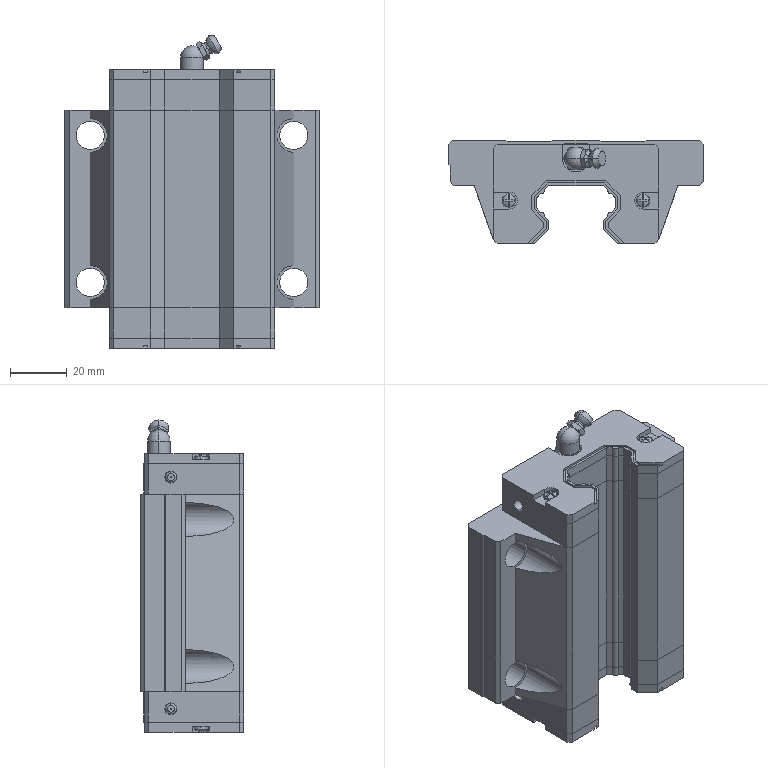Part | SolidWorks | features ICE 23, Extrusion 5, MirrorPattern 5, Fillet 4, MirrorSolid 4, Chamfer 3, RevCut 3, Dome 2, LPattern 2, Revolution 2, DeleteBody 1, LibraryFeature 1 | 6 solids | 826 faces | box 90 x 36.51 x 110.4 mm | volume 194935 mm3 | plane 567 | spline 119 | cylinder 82 | torus 25 | cone 23 | sphere 10 | commonest cylinder face diameters 2.822 x30 4.26 x12 0.575 x8 4.788 x8 10 x8 5.985 x6